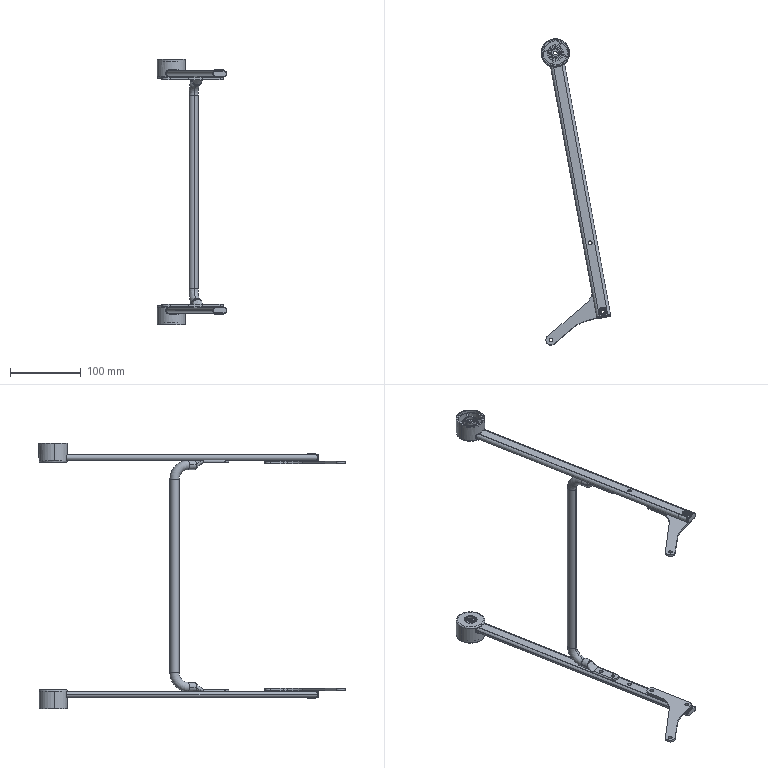Part | SolidWorks | 15 solids | 556 faces | box 98.066 x 431.233 x 374.485 mm | volume 114494 mm3 | cylinder 282 | plane 218 | spline 48 | torus 8 | commonest cylinder face diameters 5.2 x74 7.336 x24 10.049 x24 1 x12 5.326 x12 8 x12